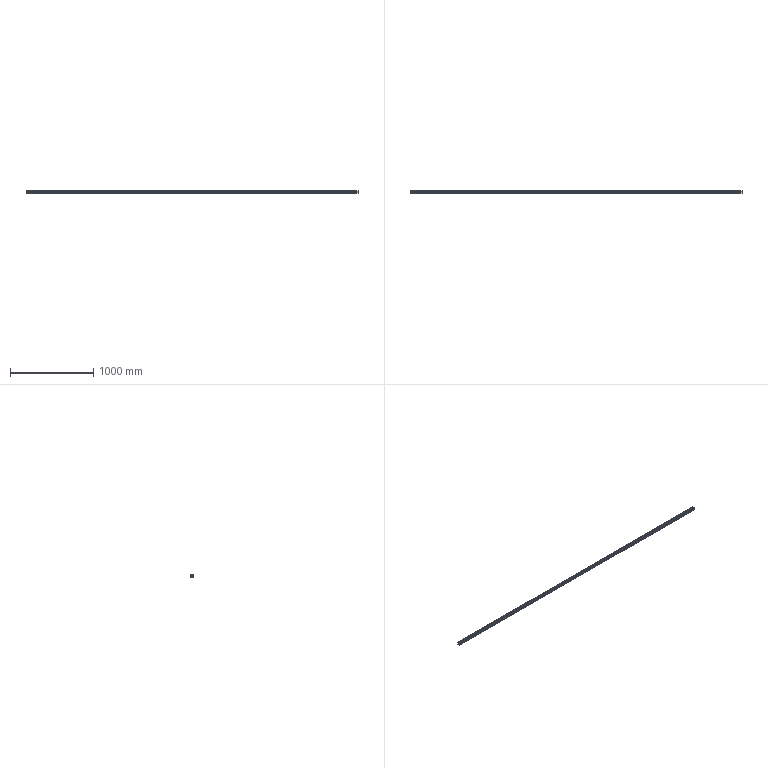Part | STEP file | _MSA35A2SS+R3980-30_30N2_(G-M61SSG-M6) | 1 solid | 434 faces | box 3980 x 29 x 34 mm | volume 3160626 mm3 | plane 230 | cylinder 204 | commonest cylinder face diameters 9 x100 14 x100 7 x4